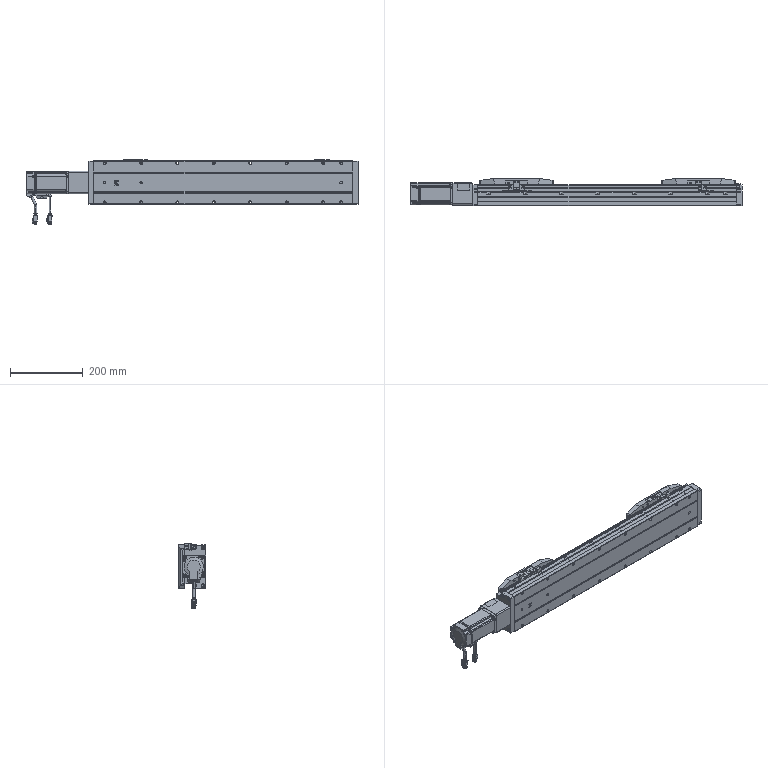Part | SolidWorks | features BaseBody 18, LPattern 1 | 19 solids | 2212 faces | box 912 x 76 x 178.533 mm | volume 5760586 mm3 | plane 1397 | cylinder 604 | cone 129 | spline 66 | torus 16 | commonest cylinder face diameters 4 x99 6 x39 8 x36 4.917 x32 5.5 x32 6.647 x32